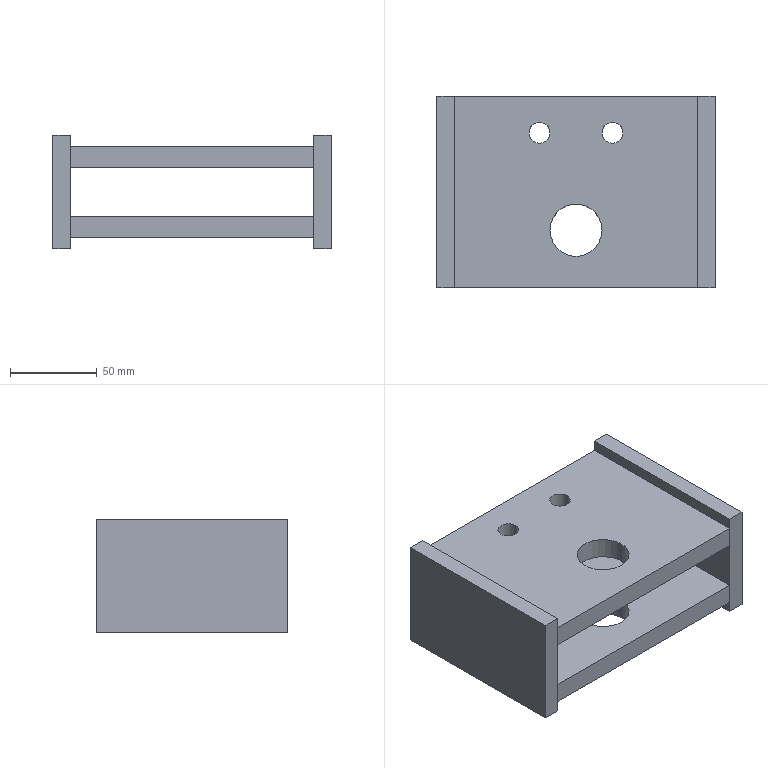Part | STEP file | Lifting fork connecting plate 2_default<machining> | 4 solids | 36 faces | box 160 x 110 x 65 mm | volume 490207 mm3 | plane 24 | cylinder 12 | commonest cylinder face diameters 12 x8 30 x4